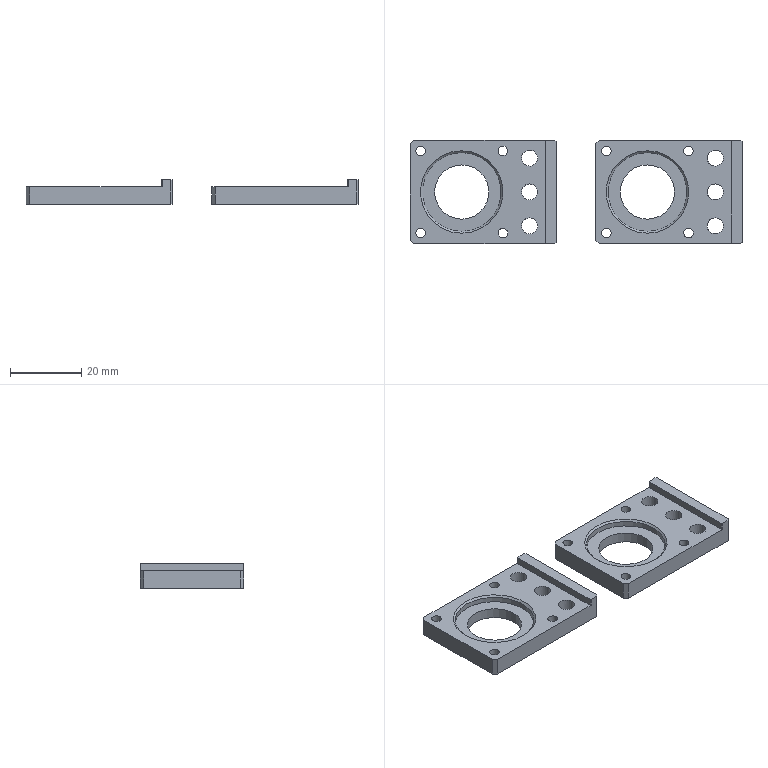Part | 2 solids | 66 faces | box 93 x 29 x 7 mm | volume 8674 mm3 | plane 38 | cylinder 26 | cone 2 | commonest cylinder face diameters 4.5 x14 2.7 x8 15.2 x2 22.1 x2